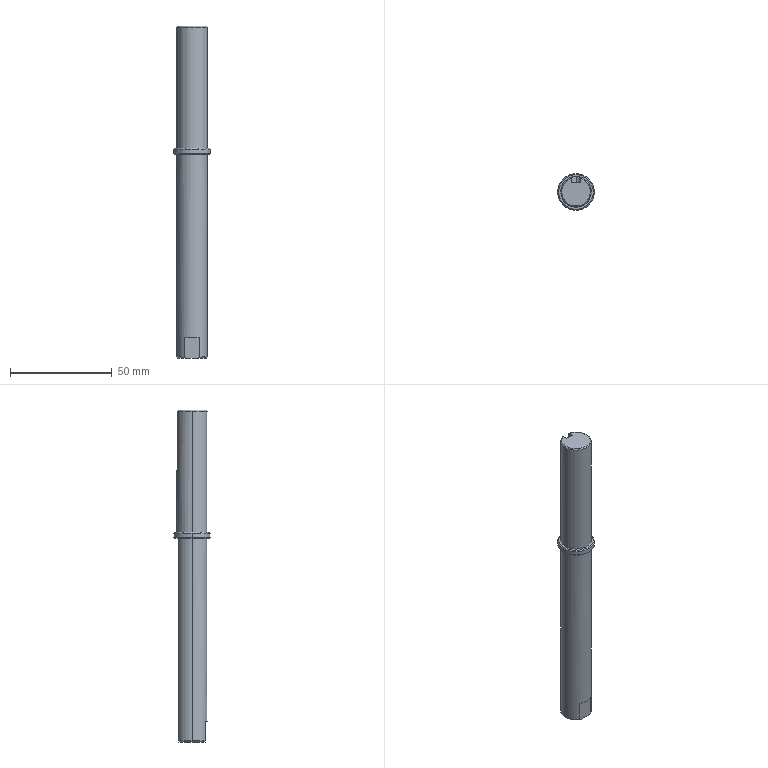Part | STEP file | 10000020500swp000-1 | 1 solid | 29 faces | box 18 x 18 x 163 mm | volume 28114 mm3 | cone 10 | plane 10 | cylinder 9 | commonest cylinder face diameters 15 x5 4 x2 18 x2
STEP:
#1=CARTESIAN_POINT('',(7.,0.,0.));
#2=VERTEX_POINT('',#1);
#3=CARTESIAN_POINT('',(2.,6.708,0.));
#4=VERTEX_POINT('',#3);
#5=CARTESIAN_POINT('',(0.,0.,0.));
#6=DIRECTION('',(0.,0.,1.));
#7=DIRECTION('',(1.,0.,0.));
#8=AXIS2_PLACEMENT_3D('',#5,#6,#7);
#9=CIRCLE('',#8,7.);
#10=EDGE_CURVE('',#2,#4,#9,.T.);
#11=ORIENTED_EDGE('',*,*,#10,.F.);
#12=CARTESIAN_POINT('',(7.5,0.,-0.5));
#13=VERTEX_POINT('',#12);
#14=CARTESIAN_POINT('',(7.,0.,0.));
#15=DIRECTION('',(0.7071,0.,-0.7071));
#16=VECTOR('',#15,1000.);
#17=LINE('',#14,#16);
#18=EDGE_CURVE('',#2,#13,#17,.T.);
#19=ORIENTED_EDGE('',*,*,#18,.T.);
#20=CARTESIAN_POINT('',(2.,7.228,-0.5));
#21=VERTEX_POINT('',#20);
#22=CARTESIAN_POINT('',(0.,0.,-0.5));
#23=DIRECTION('',(0.,0.,-1.));
#24=DIRECTION('',(1.,0.,0.));
#25=AXIS2_PLACEMENT_3D('',#22,#23,#24);
#26=CIRCLE('',#25,7.5);
#27=EDGE_CURVE('',#21,#13,#26,.T.);
#28=ORIENTED_EDGE('',*,*,#27,.F.);
#29=CARTESIAN_POINT('',(2.,6.708,0.));
#30=CARTESIAN_POINT('',(2.,6.882,-0.1664));
#31=CARTESIAN_POINT('',(2.,7.055,-0.3331));
#32=CARTESIAN_POINT('',(2.,7.228,-0.5));
#33=B_SPLINE_CURVE_WITH_KNOTS('',3,(#29,#30,#31,#32),.UNSPECIFIED.,.F.,.F.,(4,4),(0.,0.0007215),.UNSPECIFIED.);
#34=EDGE_CURVE('',#4,#21,#33,.T.);
#35=ORIENTED_EDGE('',*,*,#34,.F.);
#36=EDGE_LOOP('',(#11,#19,#28,#35));
#37=FACE_OUTER_BOUND('',#36,.T.);
#38=CARTESIAN_POINT('',(0.,0.,0.));
#39=DIRECTION('',(0.,0.,-1.));
#40=DIRECTION('',(-1.,0.,0.));
#41=AXIS2_PLACEMENT_3D('',#38,#39,#40);
#42=CONICAL_SURFACE('',#41,7.,0.7854);
#43=ADVANCED_FACE('',(#37),#42,.T.);
#44=ORIENTED_EDGE('',*,*,#18,.F.);
#45=CARTESIAN_POINT('',(-7.,0.,0.));
#46=VERTEX_POINT('',#45);
#47=CARTESIAN_POINT('',(0.,0.,0.));
#48=DIRECTION('',(0.,0.,1.));
#49=DIRECTION('',(1.,0.,0.));
#50=AXIS2_PLACEMENT_3D('',#47,#48,#49);
#51=CIRCLE('',#50,7.);
#52=EDGE_CURVE('',#46,#2,#51,.T.);
#53=ORIENTED_EDGE('',*,*,#52,.F.);
#54=CARTESIAN_POINT('',(-7.5,0.,-0.5));
#55=VERTEX_POINT('',#54);
#56=CARTESIAN_POINT('',(-7.,0.,0.));
#57=DIRECTION('',(-0.7071,0.,-0.7071));
#58=VECTOR('',#57,1000.);
#59=LINE('',#56,#58);
#60=EDGE_CURVE('',#46,#55,#59,.T.);
#61=ORIENTED_EDGE('',*,*,#60,.T.);
#62=CARTESIAN_POINT('',(0.,0.,-0.5));
#63=DIRECTION('',(0.,0.,-1.));
#64=DIRECTION('',(1.,0.,0.));
#65=AXIS2_PLACEMENT_3D('',#62,#63,#64);
#66=CIRCLE('',#65,7.5);
#67=EDGE_CURVE('',#13,#55,#66,.T.);
#68=ORIENTED_EDGE('',*,*,#67,.F.);
#69=EDGE_LOOP('',(#44,#53,#61,#68));
#70=FACE_OUTER_BOUND('',#69,.T.);
#71=CARTESIAN_POINT('',(0.,0.,0.));
#72=DIRECTION('',(0.,0.,-1.));
#73=DIRECTION('',(-1.,0.,0.));
#74=AXIS2_PLACEMENT_3D('',#71,#72,#73);
#75=CONICAL_SURFACE('',#74,7.,0.7854);
#76=ADVANCED_FACE('',(#70),#75,.T.);
#77=CARTESIAN_POINT('',(8.5,0.,-60.));
#78=VERTEX_POINT('',#77);
#79=CARTESIAN_POINT('',(-8.5,0.,-60.));
#80=VERTEX_POINT('',#79);
#81=CARTESIAN_POINT('',(0.,0.,-60.));
#82=DIRECTION('',(0.,0.,1.));
#83=DIRECTION('',(-1.,0.,0.));
#84=AXIS2_PLACEMENT_3D('',#81,#82,#83);
#85=CIRCLE('',#84,8.5);
#86=EDGE_CURVE('',#78,#80,#85,.T.);
#87=ORIENTED_EDGE('',*,*,#86,.F.);
#88=CARTESIAN_POINT('',(9.,0.,-60.5));
#89=VERTEX_POINT('',#88);
#90=CARTESIAN_POINT('',(9.,0.,-60.5));
#91=DIRECTION('',(0.7071,0.,-0.7071));
#92=VECTOR('',#91,1000.);
#93=LINE('',#90,#92);
#94=EDGE_CURVE('',#78,#89,#93,.T.);
#95=ORIENTED_EDGE('',*,*,#94,.T.);
#96=CARTESIAN_POINT('',(-9.,0.,-60.5));
#97=VERTEX_POINT('',#96);
#98=CARTESIAN_POINT('',(0.,0.,-60.5));
#99=DIRECTION('',(0.,0.,-1.));
#100=DIRECTION('',(-1.,0.,0.));
#101=AXIS2_PLACEMENT_3D('',#98,#99,#100);
#102=CIRCLE('',#101,9.);
#103=EDGE_CURVE('',#97,#89,#102,.T.);
#104=ORIENTED_EDGE('',*,*,#103,.F.);
#105=CARTESIAN_POINT('',(-9.,0.,-60.5));
#106=DIRECTION('',(-0.7071,0.,-0.7071));
#107=VECTOR('',#106,1000.);
#108=LINE('',#105,#107);
#109=EDGE_CURVE('',#80,#97,#108,.T.);
#110=ORIENTED_EDGE('',*,*,#109,.F.);
#111=EDGE_LOOP('',(#87,#95,#104,#110));
#112=FACE_OUTER_BOUND('',#111,.T.);
#113=CARTESIAN_POINT('',(0.,0.,-60.5));
#114=DIRECTION('',(0.,0.,-1.));
#115=DIRECTION('',(-1.,0.,0.));
#116=AXIS2_PLACEMENT_3D('',#113,#114,#115);
#117=CONICAL_SURFACE('',#116,9.,0.7854);
#118=ADVANCED_FACE('',(#112),#117,.T.);
#119=CARTESIAN_POINT('',(-8.5,0.,-63.));
#120=VERTEX_POINT('',#119);
#121=CARTESIAN_POINT('',(8.5,0.,-63.));
#122=VERTEX_POINT('',#121);
#123=CARTESIAN_POINT('',(0.,0.,-63.));
#124=DIRECTION('',(0.,0.,-1.));
#125=DIRECTION('',(-1.,0.,0.));
#126=AXIS2_PLACEMENT_3D('',#123,#124,#125);
#127=CIRCLE('',#126,8.5);
#128=EDGE_CURVE('',#120,#122,#127,.T.);
#129=ORIENTED_EDGE('',*,*,#128,.F.);
#130=CARTESIAN_POINT('',(-9.,0.,-62.5));
#131=VERTEX_POINT('',#130);
#132=CARTESIAN_POINT('',(-8.5,0.,-63.));
#133=DIRECTION('',(-0.7071,0.,0.7071));
#134=VECTOR('',#133,1000.);
#135=LINE('',#132,#134);
#136=EDGE_CURVE('',#120,#131,#135,.T.);
#137=ORIENTED_EDGE('',*,*,#136,.T.);
#138=CARTESIAN_POINT('',(9.,0.,-62.5));
#139=VERTEX_POINT('',#138);
#140=CARTESIAN_POINT('',(0.,0.,-62.5));
#141=DIRECTION('',(0.,0.,1.));
#142=DIRECTION('',(-1.,0.,0.));
#143=AXIS2_PLACEMENT_3D('',#140,#141,#142);
#144=CIRCLE('',#143,9.);
#145=EDGE_CURVE('',#139,#131,#144,.T.);
#146=ORIENTED_EDGE('',*,*,#145,.F.);
#147=CARTESIAN_POINT('',(8.5,0.,-63.));
#148=DIRECTION('',(0.7071,0.,0.7071));
#149=VECTOR('',#148,1000.);
#150=LINE('',#147,#149);
#151=EDGE_CURVE('',#122,#139,#150,.T.);
#152=ORIENTED_EDGE('',*,*,#151,.F.);
#153=EDGE_LOOP('',(#129,#137,#146,#152));
#154=FACE_OUTER_BOUND('',#153,.T.);
#155=CARTESIAN_POINT('',(0.,0.,-63.));
#156=DIRECTION('',(0.,0.,1.));
#157=DIRECTION('',(1.,0.,0.));
#158=AXIS2_PLACEMENT_3D('',#155,#156,#157);
#159=CONICAL_SURFACE('',#158,8.5,0.7854);
#160=ADVANCED_FACE('',(#154),#159,.T.);
#161=CARTESIAN_POINT('',(7.,0.,-163.));
#162=VERTEX_POINT('',#161);
#163=CARTESIAN_POINT('',(2.598,-6.5,-163.));
#164=VERTEX_POINT('',#163);
#165=CARTESIAN_POINT('',(0.,0.,-163.));
#166=DIRECTION('',(0.,0.,-1.));
#167=DIRECTION('',(-1.,0.,0.));
#168=AXIS2_PLACEMENT_3D('',#165,#166,#167);
#169=CIRCLE('',#168,7.);
#170=EDGE_CURVE('',#162,#164,#169,.T.);
#171=ORIENTED_EDGE('',*,*,#170,.F.);
#172=CARTESIAN_POINT('',(7.5,0.,-162.5));
#173=VERTEX_POINT('',#172);
#174=CARTESIAN_POINT('',(7.,0.,-163.));
#175=DIRECTION('',(0.7071,0.,0.7071));
#176=VECTOR('',#175,1000.);
#177=LINE('',#174,#176);
#178=EDGE_CURVE('',#162,#173,#177,.T.);
#179=ORIENTED_EDGE('',*,*,#178,.T.);
#180=CARTESIAN_POINT('',(3.742,-6.5,-162.5));
#181=VERTEX_POINT('',#180);
#182=CARTESIAN_POINT('',(0.,0.,-162.5));
#183=DIRECTION('',(0.,0.,1.));
#184=DIRECTION('',(-1.,0.,0.));
#185=AXIS2_PLACEMENT_3D('',#182,#183,#184);
#186=CIRCLE('',#185,7.5);
#187=EDGE_CURVE('',#181,#173,#186,.T.);
#188=ORIENTED_EDGE('',*,*,#187,.F.);
#189=CARTESIAN_POINT('',(2.598,-6.5,-163.));
#190=CARTESIAN_POINT('',(2.991,-6.5,-162.854));
#191=CARTESIAN_POINT('',(3.371,-6.5,-162.685));
#192=CARTESIAN_POINT('',(3.742,-6.5,-162.5));
#193=B_SPLINE_CURVE_WITH_KNOTS('',3,(#189,#190,#191,#192),.UNSPECIFIED.,.F.,.F.,(4,4),(0.02116,0.02241),.UNSPECIFIED.);
#194=EDGE_CURVE('',#164,#181,#193,.T.);
#195=ORIENTED_EDGE('',*,*,#194,.F.);
#196=EDGE_LOOP('',(#171,#179,#188,#195));
#197=FACE_OUTER_BOUND('',#196,.T.);
#198=CARTESIAN_POINT('',(0.,0.,-163.));
#199=DIRECTION('',(0.,0.,1.));
#200=DIRECTION('',(1.,0.,0.));
#201=AXIS2_PLACEMENT_3D('',#198,#199,#200);
#202=CONICAL_SURFACE('',#201,7.,0.7854);
#203=ADVANCED_FACE('',(#197),#202,.T.);
#204=CARTESIAN_POINT('',(0.,7.5,-30.));
#205=VERTEX_POINT('',#204);
#206=CARTESIAN_POINT('',(2.,7.228,-28.));
#207=VERTEX_POINT('',#206);
#208=CARTESIAN_POINT('',(0.,7.5,-30.));
#209=CARTESIAN_POINT('',(0.131,7.5,-30.));
#210=CARTESIAN_POINT('',(0.2641,7.496,-29.987));
#211=CARTESIAN_POINT('',(0.5209,7.483,-29.935));
#212=CARTESIAN_POINT('',(0.6458,7.473,-29.897));
#213=CARTESIAN_POINT('',(1.01,7.436,-29.746));
#214=CARTESIAN_POINT('',(1.229,7.401,-29.599));
#215=CARTESIAN_POINT('',(1.507,7.348,-29.322));
#216=CARTESIAN_POINT('',(1.589,7.33,-29.221));
#217=CARTESIAN_POINT('',(1.734,7.297,-29.006));
#218=CARTESIAN_POINT('',(1.797,7.282,-28.889));
#219=CARTESIAN_POINT('',(1.897,7.256,-28.648));
#220=CARTESIAN_POINT('',(1.935,7.246,-28.523));
#221=CARTESIAN_POINT('',(1.987,7.232,-28.265));
#222=CARTESIAN_POINT('',(2.,7.228,-28.133));
#223=CARTESIAN_POINT('',(2.,7.228,-28.));
#224=B_SPLINE_CURVE_WITH_KNOTS('',3,(#208,#209,#210,#211,#212,#213,#214,#215,#216,#217,#218,#219,#220,#221,#222,#223),.UNSPECIFIED.,.F.,.F.,(4,2,2,2,2,2,2,4),(0.003142,0.003534,0.003926,0.00471,0.005103,0.005495,0.005887,0.006279),.UNSPECIFIED.);
#225=EDGE_CURVE('',#205,#207,#224,.T.);
#226=ORIENTED_EDGE('',*,*,#225,.F.);
#227=CARTESIAN_POINT('',(0.,4.5,-30.));
#228=VERTEX_POINT('',#227);
#229=CARTESIAN_POINT('',(0.,9.,-30.));
#230=DIRECTION('',(0.,-1.,0.));
#231=VECTOR('',#230,1000.);
#232=LINE('',#229,#231);
#233=EDGE_CURVE('',#205,#228,#232,.T.);
#234=ORIENTED_EDGE('',*,*,#233,.T.);
#235=CARTESIAN_POINT('',(2.,4.5,-28.));
#236=VERTEX_POINT('',#235);
#237=CARTESIAN_POINT('',(0.,4.5,-28.));
#238=DIRECTION('',(0.,1.,0.));
#239=DIRECTION('',(0.,0.,1.));
#240=AXIS2_PLACEMENT_3D('',#237,#238,#239);
#241=CIRCLE('',#240,2.);
#242=EDGE_CURVE('',#236,#228,#241,.T.);
#243=ORIENTED_EDGE('',*,*,#242,.F.);
#244=CARTESIAN_POINT('',(2.,9.,-28.));
#245=DIRECTION('',(0.,-1.,0.));
#246=VECTOR('',#245,1000.);
#247=LINE('',#244,#246);
#248=EDGE_CURVE('',#207,#236,#247,.T.);
#249=ORIENTED_EDGE('',*,*,#248,.F.);
#250=EDGE_LOOP('',(#226,#234,#243,#249));
#251=FACE_OUTER_BOUND('',#250,.T.);
#252=CARTESIAN_POINT('',(0.,9.,-28.));
#253=DIRECTION('',(0.,-1.,0.));
#254=DIRECTION('',(0.,0.,-1.));
#255=AXIS2_PLACEMENT_3D('',#252,#253,#254);
#256=CYLINDRICAL_SURFACE('',#255,2.);
#257=ADVANCED_FACE('',(#251),#256,.F.);
#258=ORIENTED_EDGE('',*,*,#145,.T.);
#259=CARTESIAN_POINT('',(-9.,0.,-63.));
#260=DIRECTION('',(0.,0.,1.));
#261=VECTOR('',#260,1000.);
#262=LINE('',#259,#261);
#263=EDGE_CURVE('',#131,#97,#262,.T.);
#264=ORIENTED_EDGE('',*,*,#263,.T.);
#265=ORIENTED_EDGE('',*,*,#103,.T.);
#266=CARTESIAN_POINT('',(9.,0.,-63.));
#267=DIRECTION('',(0.,0.,1.));
#268=VECTOR('',#267,1000.);
#269=LINE('',#266,#268);
#270=EDGE_CURVE('',#139,#89,#269,.T.);
#271=ORIENTED_EDGE('',*,*,#270,.F.);
#272=EDGE_LOOP('',(#258,#264,#265,#271));
#273=FACE_OUTER_BOUND('',#272,.T.);
#274=CARTESIAN_POINT('',(0.,0.,-63.));
#275=DIRECTION('',(0.,0.,1.));
#276=DIRECTION('',(1.,0.,0.));
#277=AXIS2_PLACEMENT_3D('',#274,#275,#276);
#278=CYLINDRICAL_SURFACE('',#277,9.);
#279=ADVANCED_FACE('',(#273),#278,.T.);
#280=CARTESIAN_POINT('',(-3.742,6.5,-162.5));
#281=VERTEX_POINT('',#280);
#282=CARTESIAN_POINT('',(-7.5,0.,-162.5));
#283=VERTEX_POINT('',#282);
#284=CARTESIAN_POINT('',(0.,0.,-162.5));
#285=DIRECTION('',(0.,0.,1.));
#286=DIRECTION('',(-1.,0.,0.));
#287=AXIS2_PLACEMENT_3D('',#284,#285,#286);
#288=CIRCLE('',#287,7.5);
#289=EDGE_CURVE('',#281,#283,#288,.T.);
#290=ORIENTED_EDGE('',*,*,#289,.T.);
#291=CARTESIAN_POINT('',(-7.5,0.,-63.));
#292=VERTEX_POINT('',#291);
#293=CARTESIAN_POINT('',(-7.5,0.,-163.));
#294=DIRECTION('',(0.,0.,1.));
#295=VECTOR('',#294,1000.);
#296=LINE('',#293,#295);
#297=EDGE_CURVE('',#283,#292,#296,.T.);
#298=ORIENTED_EDGE('',*,*,#297,.T.);
#299=CARTESIAN_POINT('',(-3.742,6.5,-63.));
#300=VERTEX_POINT('',#299);
#301=CARTESIAN_POINT('',(0.,0.,-63.));
#302=DIRECTION('',(0.,0.,-1.));
#303=DIRECTION('',(-1.,0.,0.));
#304=AXIS2_PLACEMENT_3D('',#301,#302,#303);
#305=CIRCLE('',#304,7.5);
#306=EDGE_CURVE('',#292,#300,#305,.T.);
#307=ORIENTED_EDGE('',*,*,#306,.T.);
#308=CARTESIAN_POINT('',(-3.742,6.5,-163.));
#309=DIRECTION('',(0.,0.,1.));
#310=VECTOR('',#309,1000.);
#311=LINE('',#308,#310);
#312=EDGE_CURVE('',#281,#300,#311,.T.);
#313=ORIENTED_EDGE('',*,*,#312,.F.);
#314=EDGE_LOOP('',(#290,#298,#307,#313));
#315=FACE_OUTER_BOUND('',#314,.T.);
#316=CARTESIAN_POINT('',(0.,0.,-163.));
#317=DIRECTION('',(0.,0.,1.));
#318=DIRECTION('',(1.,0.,0.));
#319=AXIS2_PLACEMENT_3D('',#316,#317,#318);
#320=CYLINDRICAL_SURFACE('',#319,7.5);
#321=ADVANCED_FACE('',(#315),#320,.T.);
#322=ORIENTED_EDGE('',*,*,#297,.F.);
#323=CARTESIAN_POINT('',(-3.742,-6.5,-162.5));
#324=VERTEX_POINT('',#323);
#325=CARTESIAN_POINT('',(0.,0.,-162.5));
#326=DIRECTION('',(0.,0.,1.));
#327=DIRECTION('',(-1.,0.,0.));
#328=AXIS2_PLACEMENT_3D('',#325,#326,#327);
#329=CIRCLE('',#328,7.5);
#330=EDGE_CURVE('',#283,#324,#329,.T.);
#331=ORIENTED_EDGE('',*,*,#330,.T.);
#332=CARTESIAN_POINT('',(-3.742,-6.5,-153.));
#333=VERTEX_POINT('',#332);
#334=CARTESIAN_POINT('',(-3.742,-6.5,-163.));
#335=DIRECTION('',(0.,0.,1.));
#336=VECTOR('',#335,1000.);
#337=LINE('',#334,#336);
#338=EDGE_CURVE('',#324,#333,#337,.T.);
#339=ORIENTED_EDGE('',*,*,#338,.T.);
#340=CARTESIAN_POINT('',(3.742,-6.5,-153.));
#341=VERTEX_POINT('',#340);
#342=CARTESIAN_POINT('',(0.,0.,-153.));
#343=DIRECTION('',(0.,0.,1.));
#344=DIRECTION('',(1.,0.,0.));
#345=AXIS2_PLACEMENT_3D('',#342,#343,#344);
#346=CIRCLE('',#345,7.5);
#347=EDGE_CURVE('',#333,#341,#346,.T.);
#348=ORIENTED_EDGE('',*,*,#347,.T.);
#349=CARTESIAN_POINT('',(3.742,-6.5,-163.));
#350=DIRECTION('',(0.,0.,-1.));
#351=VECTOR('',#350,1000.);
#352=LINE('',#349,#351);
#353=EDGE_CURVE('',#341,#181,#352,.T.);
#354=ORIENTED_EDGE('',*,*,#353,.T.);
#355=ORIENTED_EDGE('',*,*,#187,.T.);
#356=CARTESIAN_POINT('',(7.5,0.,-63.));
#357=VERTEX_POINT('',#356);
#358=CARTESIAN_POINT('',(7.5,0.,-163.));
#359=DIRECTION('',(0.,0.,1.));
#360=VECTOR('',#359,1000.);
#361=LINE('',#358,#360);
#362=EDGE_CURVE('',#173,#357,#361,.T.);
#363=ORIENTED_EDGE('',*,*,#362,.T.);
#364=CARTESIAN_POINT('',(0.,0.,-63.));
#365=DIRECTION('',(0.,0.,-1.));
#366=DIRECTION('',(-1.,0.,0.));
#367=AXIS2_PLACEMENT_3D('',#364,#365,#366);
#368=CIRCLE('',#367,7.5);
#369=EDGE_CURVE('',#357,#292,#368,.T.);
#370=ORIENTED_EDGE('',*,*,#369,.T.);
#371=EDGE_LOOP('',(#322,#331,#339,#348,#354,#355,#363,#370));
#372=FACE_OUTER_BOUND('',#371,.T.);
#373=CARTESIAN_POINT('',(0.,0.,-163.));
#374=DIRECTION('',(0.,0.,1.));
#375=DIRECTION('',(1.,0.,0.));
#376=AXIS2_PLACEMENT_3D('',#373,#374,#375);
#377=CYLINDRICAL_SURFACE('',#376,7.5);
#378=ADVANCED_FACE('',(#372),#377,.T.);
#379=CARTESIAN_POINT('',(7.5,0.,-60.));
#380=VERTEX_POINT('',#379);
#381=CARTESIAN_POINT('',(-7.5,0.,-60.));
#382=VERTEX_POINT('',#381);
#383=CARTESIAN_POINT('',(0.,0.,-60.));
#384=DIRECTION('',(0.,0.,1.));
#385=DIRECTION('',(-1.,0.,0.));
#386=AXIS2_PLACEMENT_3D('',#383,#384,#385);
#387=CIRCLE('',#386,7.5);
#388=EDGE_CURVE('',#380,#382,#387,.T.);
#389=ORIENTED_EDGE('',*,*,#388,.T.);
#390=CARTESIAN_POINT('',(-7.5,0.,-60.));
#391=DIRECTION('',(0.,0.,1.));
#392=VECTOR('',#391,1000.);
#393=LINE('',#390,#392);
#394=EDGE_CURVE('',#382,#55,#393,.T.);
#395=ORIENTED_EDGE('',*,*,#394,.T.);
#396=CARTESIAN_POINT('',(-2.,7.228,-0.5));
#397=VERTEX_POINT('',#396);
#398=CARTESIAN_POINT('',(0.,0.,-0.5));
#399=DIRECTION('',(0.,0.,-1.));
#400=DIRECTION('',(1.,0.,0.));
#401=AXIS2_PLACEMENT_3D('',#398,#399,#400);
#402=CIRCLE('',#401,7.5);
#403=EDGE_CURVE('',#55,#397,#402,.T.);
#404=ORIENTED_EDGE('',*,*,#403,.T.);
#405=CARTESIAN_POINT('',(-2.,7.228,-28.));
#406=VERTEX_POINT('',#405);
#407=CARTESIAN_POINT('',(-2.,7.228,-60.));
#408=DIRECTION('',(0.,0.,-1.));
#409=VECTOR('',#408,1000.);
#410=LINE('',#407,#409);
#411=EDGE_CURVE('',#397,#406,#410,.T.);
#412=ORIENTED_EDGE('',*,*,#411,.T.);
#413=CARTESIAN_POINT('',(-2.,7.228,-28.));
#414=CARTESIAN_POINT('',(-2.,7.228,-28.133));
#415=CARTESIAN_POINT('',(-1.987,7.232,-28.263));
#416=CARTESIAN_POINT('',(-1.936,7.246,-28.52));
#417=CARTESIAN_POINT('',(-1.897,7.256,-28.647));
#418=CARTESIAN_POINT('',(-1.796,7.282,-28.889));
#419=CARTESIAN_POINT('',(-1.735,7.297,-29.004));
#420=CARTESIAN_POINT('',(-1.59,7.33,-29.221));
#421=CARTESIAN_POINT('',(-1.505,7.348,-29.323));
#422=CARTESIAN_POINT('',(-1.23,7.401,-29.598));
#423=CARTESIAN_POINT('',(-1.008,7.436,-29.747));
#424=CARTESIAN_POINT('',(-0.6467,7.473,-29.897));
#425=CARTESIAN_POINT('',(-0.52,7.483,-29.936));
#426=CARTESIAN_POINT('',(-0.2614,7.497,-29.987));
#427=CARTESIAN_POINT('',(-0.1312,7.5,-30.));
#428=CARTESIAN_POINT('',(0.,7.5,-30.));
#429=B_SPLINE_CURVE_WITH_KNOTS('',3,(#413,#414,#415,#416,#417,#418,#419,#420,#421,#422,#423,#424,#425,#426,#427,#428),.UNSPECIFIED.,.F.,.F.,(4,2,2,2,2,2,2,4),(0.,0.0003927,0.0007854,0.001178,0.001571,0.002356,0.002749,0.003142),.UNSPECIFIED.);
#430=EDGE_CURVE('',#406,#205,#429,.T.);
#431=ORIENTED_EDGE('',*,*,#430,.T.);
#432=ORIENTED_EDGE('',*,*,#225,.T.);
#433=CARTESIAN_POINT('',(2.,7.228,-60.));
#434=DIRECTION('',(0.,0.,1.));
#435=VECTOR('',#434,1000.);
#436=LINE('',#433,#435);
#437=EDGE_CURVE('',#207,#21,#436,.T.);
#438=ORIENTED_EDGE('',*,*,#437,.T.);
#439=ORIENTED_EDGE('',*,*,#27,.T.);
#440=CARTESIAN_POINT('',(7.5,0.,-60.));
#441=DIRECTION('',(0.,0.,1.));
#442=VECTOR('',#441,1000.);
#443=LINE('',#440,#442);
#444=EDGE_CURVE('',#380,#13,#443,.T.);
#445=ORIENTED_EDGE('',*,*,#444,.F.);
#446=EDGE_LOOP('',(#389,#395,#404,#412,#431,#432,#438,#439,#445));
#447=FACE_OUTER_BOUND('',#446,.T.);
#448=CARTESIAN_POINT('',(0.,0.,-60.));
#449=DIRECTION('',(0.,0.,1.));
#450=DIRECTION('',(1.,0.,0.));
#451=AXIS2_PLACEMENT_3D('',#448,#449,#450);
#452=CYLINDRICAL_SURFACE('',#451,7.5);
#453=ADVANCED_FACE('',(#447),#452,.T.);
#454=CARTESIAN_POINT('',(-2.598,-6.5,-163.));
#455=VERTEX_POINT('',#454);
#456=CARTESIAN_POINT('',(-3.742,-6.5,-162.5));
#457=CARTESIAN_POINT('',(-3.369,-6.5,-162.686));
#458=CARTESIAN_POINT('',(-2.989,-6.5,-162.855));
#459=CARTESIAN_POINT('',(-2.598,-6.5,-163.));
#460=B_SPLINE_CURVE_WITH_KNOTS('',3,(#456,#457,#458,#459),.UNSPECIFIED.,.F.,.F.,(4,4),(0.01459,0.01584),.UNSPECIFIED.);
#461=EDGE_CURVE('',#324,#455,#460,.T.);
#462=ORIENTED_EDGE('',*,*,#461,.F.);
#463=ORIENTED_EDGE('',*,*,#330,.F.);
#464=ORIENTED_EDGE('',*,*,#289,.F.);
#465=CARTESIAN_POINT('',(-2.598,6.5,-163.));
#466=VERTEX_POINT('',#465);
#467=CARTESIAN_POINT('',(-2.598,6.5,-163.));
#468=CARTESIAN_POINT('',(-2.989,6.5,-162.855));
#469=CARTESIAN_POINT('',(-3.369,6.5,-162.686));
#470=CARTESIAN_POINT('',(-3.742,6.5,-162.5));
#471=B_SPLINE_CURVE_WITH_KNOTS('',3,(#467,#468,#469,#470),.UNSPECIFIED.,.F.,.F.,(4,4),(0.,0.001248),.UNSPECIFIED.);
#472=EDGE_CURVE('',#466,#281,#471,.T.);
#473=ORIENTED_EDGE('',*,*,#472,.F.);
#474=CARTESIAN_POINT('',(0.,0.,-163.));
#475=DIRECTION('',(0.,0.,-1.));
#476=DIRECTION('',(-1.,0.,0.));
#477=AXIS2_PLACEMENT_3D('',#474,#475,#476);
#478=CIRCLE('',#477,7.);
#479=EDGE_CURVE('',#455,#466,#478,.T.);
#480=ORIENTED_EDGE('',*,*,#479,.F.);
#481=EDGE_LOOP('',(#462,#463,#464,#473,#480));
#482=FACE_OUTER_BOUND('',#481,.T.);
#483=CARTESIAN_POINT('',(0.,0.,-163.));
#484=DIRECTION('',(0.,0.,1.));
#485=DIRECTION('',(1.,0.,0.));
#486=AXIS2_PLACEMENT_3D('',#483,#484,#485);
#487=CONICAL_SURFACE('',#486,7.,0.7854);
#488=ADVANCED_FACE('',(#482),#487,.T.);
#489=ORIENTED_EDGE('',*,*,#394,.F.);
#490=CARTESIAN_POINT('',(0.,0.,-60.));
#491=DIRECTION('',(0.,0.,1.));
#492=DIRECTION('',(-1.,0.,0.));
#493=AXIS2_PLACEMENT_3D('',#490,#491,#492);
#494=CIRCLE('',#493,7.5);
#495=EDGE_CURVE('',#382,#380,#494,.T.);
#496=ORIENTED_EDGE('',*,*,#495,.T.);
#497=ORIENTED_EDGE('',*,*,#444,.T.);
#498=ORIENTED_EDGE('',*,*,#67,.T.);
#499=EDGE_LOOP('',(#489,#496,#497,#498));
#500=FACE_OUTER_BOUND('',#499,.T.);
#501=CARTESIAN_POINT('',(0.,0.,-60.));
#502=DIRECTION('',(0.,0.,1.));
#503=DIRECTION('',(1.,0.,0.));
#504=AXIS2_PLACEMENT_3D('',#501,#502,#503);
#505=CYLINDRICAL_SURFACE('',#504,7.5);
#506=ADVANCED_FACE('',(#500),#505,.T.);
#507=CARTESIAN_POINT('',(-2.,4.5,0.));
#508=VERTEX_POINT('',#507);
#509=CARTESIAN_POINT('',(-2.,6.708,0.));
#510=VERTEX_POINT('',#509);
#511=CARTESIAN_POINT('',(-2.,0.,0.));
#512=DIRECTION('',(0.,1.,0.));
#513=VECTOR('',#512,1000.);
#514=LINE('',#511,#513);
#515=EDGE_CURVE('',#508,#510,#514,.T.);
#516=ORIENTED_EDGE('',*,*,#515,.T.);
#517=CARTESIAN_POINT('',(0.,0.,0.));
#518=DIRECTION('',(0.,0.,1.));
#519=DIRECTION('',(1.,0.,0.));
#520=AXIS2_PLACEMENT_3D('',#517,#518,#519);
#521=CIRCLE('',#520,7.);
#522=EDGE_CURVE('',#510,#46,#521,.T.);
#523=ORIENTED_EDGE('',*,*,#522,.T.);
#524=ORIENTED_EDGE('',*,*,#52,.T.);
#525=ORIENTED_EDGE('',*,*,#10,.T.);
#526=CARTESIAN_POINT('',(2.,4.5,0.));
#527=VERTEX_POINT('',#526);
#528=CARTESIAN_POINT('',(2.,0.,0.));
#529=DIRECTION('',(0.,-1.,0.));
#530=VECTOR('',#529,1000.);
#531=LINE('',#528,#530);
#532=EDGE_CURVE('',#4,#527,#531,.T.);
#533=ORIENTED_EDGE('',*,*,#532,.T.);
#534=CARTESIAN_POINT('',(0.,4.5,0.));
#535=DIRECTION('',(-1.,0.,0.));
#536=VECTOR('',#535,1000.);
#537=LINE('',#534,#536);
#538=EDGE_CURVE('',#527,#508,#537,.T.);
#539=ORIENTED_EDGE('',*,*,#538,.T.);
#540=EDGE_LOOP('',(#516,#523,#524,#525,#533,#539));
#541=FACE_OUTER_BOUND('',#540,.T.);
#542=CARTESIAN_POINT('',(0.,0.,0.));
#543=DIRECTION('',(0.,0.,1.));
#544=DIRECTION('',(1.,0.,0.));
#545=AXIS2_PLACEMENT_3D('',#542,#543,#544);
#546=PLANE('',#545);
#547=ADVANCED_FACE('',(#541),#546,.T.);
#548=ORIENTED_EDGE('',*,*,#362,.F.);
#549=CARTESIAN_POINT('',(3.742,6.5,-162.5));
#550=VERTEX_POINT('',#549);
#551=CARTESIAN_POINT('',(0.,0.,-162.5));
#552=DIRECTION('',(0.,0.,1.));
#553=DIRECTION('',(-1.,0.,0.));
#554=AXIS2_PLACEMENT_3D('',#551,#552,#553);
#555=CIRCLE('',#554,7.5);
#556=EDGE_CURVE('',#173,#550,#555,.T.);
#557=ORIENTED_EDGE('',*,*,#556,.T.);
#558=CARTESIAN_POINT('',(3.742,6.5,-63.));
#559=VERTEX_POINT('',#558);
#560=CARTESIAN_POINT('',(3.742,6.5,-163.));
#561=DIRECTION('',(0.,0.,-1.));
#562=VECTOR('',#561,1000.);
#563=LINE('',#560,#562);
#564=EDGE_CURVE('',#559,#550,#563,.T.);
#565=ORIENTED_EDGE('',*,*,#564,.F.);
#566=CARTESIAN_POINT('',(0.,0.,-63.));
#567=DIRECTION('',(0.,0.,-1.));
#568=DIRECTION('',(-1.,0.,0.));
#569=AXIS2_PLACEMENT_3D('',#566,#567,#568);
#570=CIRCLE('',#569,7.5);
#571=EDGE_CURVE('',#559,#357,#570,.T.);
#572=ORIENTED_EDGE('',*,*,#571,.T.);
#573=EDGE_LOOP('',(#548,#557,#565,#572));
#574=FACE_OUTER_BOUND('',#573,.T.);
#575=CARTESIAN_POINT('',(0.,0.,-163.));
#576=DIRECTION('',(0.,0.,1.));
#577=DIRECTION('',(1.,0.,0.));
#578=AXIS2_PLACEMENT_3D('',#575,#576,#577);
#579=CYLINDRICAL_SURFACE('',#578,7.5);
#580=ADVANCED_FACE('',(#574),#579,.T.);
#581=CARTESIAN_POINT('',(-15.,-6.5,-163.));
#582=DIRECTION('',(1.,0.,0.));
#583=VECTOR('',#582,1000.);
#584=LINE('',#581,#583);
#585=EDGE_CURVE('',#455,#164,#584,.T.);
#586=ORIENTED_EDGE('',*,*,#585,.F.);
#587=ORIENTED_EDGE('',*,*,#479,.T.);
#588=CARTESIAN_POINT('',(2.598,6.5,-163.));
#589=VERTEX_POINT('',#588);
#590=CARTESIAN_POINT('',(0.,6.5,-163.));
#591=DIRECTION('',(1.,0.,0.));
#592=VECTOR('',#591,1000.);
#593=LINE('',#590,#592);
#594=EDGE_CURVE('',#466,#589,#593,.T.);
#595=ORIENTED_EDGE('',*,*,#594,.T.);
#596=CARTESIAN_POINT('',(0.,0.,-163.));
#597=DIRECTION('',(0.,0.,-1.));
#598=DIRECTION('',(-1.,0.,0.));
#599=AXIS2_PLACEMENT_3D('',#596,#597,#598);
#600=CIRCLE('',#599,7.);
#601=EDGE_CURVE('',#589,#162,#600,.T.);
#602=ORIENTED_EDGE('',*,*,#601,.T.);
#603=ORIENTED_EDGE('',*,*,#170,.T.);
#604=EDGE_LOOP('',(#586,#587,#595,#602,#603));
#605=FACE_OUTER_BOUND('',#604,.T.);
#606=CARTESIAN_POINT('',(0.,0.,-163.));
#607=DIRECTION('',(0.,0.,-1.));
#608=DIRECTION('',(-1.,0.,0.));
#609=AXIS2_PLACEMENT_3D('',#606,#607,#608);
#610=PLANE('',#609);
#611=ADVANCED_FACE('',(#605),#610,.T.);
#612=ORIENTED_EDGE('',*,*,#263,.F.);
#613=CARTESIAN_POINT('',(0.,0.,-62.5));
#614=DIRECTION('',(0.,0.,1.));
#615=DIRECTION('',(-1.,0.,0.));
#616=AXIS2_PLACEMENT_3D('',#613,#614,#615);
#617=CIRCLE('',#616,9.);
#618=EDGE_CURVE('',#131,#139,#617,.T.);
#619=ORIENTED_EDGE('',*,*,#618,.T.);
#620=ORIENTED_EDGE('',*,*,#270,.T.);
#621=CARTESIAN_POINT('',(0.,0.,-60.5));
#622=DIRECTION('',(0.,0.,-1.));
#623=DIRECTION('',(-1.,0.,0.));
#624=AXIS2_PLACEMENT_3D('',#621,#622,#623);
#625=CIRCLE('',#624,9.);
#626=EDGE_CURVE('',#89,#97,#625,.T.);
#627=ORIENTED_EDGE('',*,*,#626,.T.);
#628=EDGE_LOOP('',(#612,#619,#620,#627));
#629=FACE_OUTER_BOUND('',#628,.T.);
#630=CARTESIAN_POINT('',(0.,0.,-63.));
#631=DIRECTION('',(0.,0.,1.));
#632=DIRECTION('',(1.,0.,0.));
#633=AXIS2_PLACEMENT_3D('',#630,#631,#632);
#634=CYLINDRICAL_SURFACE('',#633,9.);
#635=ADVANCED_FACE('',(#629),#634,.T.);
#636=CARTESIAN_POINT('',(0.,0.,-63.));
#637=DIRECTION('',(0.,0.,-1.));
#638=DIRECTION('',(-1.,0.,0.));
#639=AXIS2_PLACEMENT_3D('',#636,#637,#638);
#640=CIRCLE('',#639,8.5);
#641=EDGE_CURVE('',#122,#120,#640,.T.);
#642=ORIENTED_EDGE('',*,*,#641,.T.);
#643=ORIENTED_EDGE('',*,*,#128,.T.);
#644=EDGE_LOOP('',(#642,#643));
#645=FACE_OUTER_BOUND('',#644,.T.);
#646=CARTESIAN_POINT('',(-5.,6.5,-63.));
#647=DIRECTION('',(1.,0.,0.));
#648=VECTOR('',#647,1000.);
#649=LINE('',#646,#648);
#650=EDGE_CURVE('',#300,#559,#649,.T.);
#651=ORIENTED_EDGE('',*,*,#650,.F.);
#652=ORIENTED_EDGE('',*,*,#306,.F.);
#653=ORIENTED_EDGE('',*,*,#369,.F.);
#654=ORIENTED_EDGE('',*,*,#571,.F.);
#655=EDGE_LOOP('',(#651,#652,#653,#654));
#656=FACE_BOUND('',#655,.T.);
#657=CARTESIAN_POINT('',(0.,0.,-63.));
#658=DIRECTION('',(0.,0.,-1.));
#659=DIRECTION('',(-1.,0.,0.));
#660=AXIS2_PLACEMENT_3D('',#657,#658,#659);
#661=PLANE('',#660);
#662=ADVANCED_FACE('',(#645,#656),#661,.T.);
#663=CARTESIAN_POINT('',(0.,0.,-60.));
#664=DIRECTION('',(0.,0.,1.));
#665=DIRECTION('',(-1.,0.,0.));
#666=AXIS2_PLACEMENT_3D('',#663,#664,#665);
#667=CIRCLE('',#666,8.5);
#668=EDGE_CURVE('',#80,#78,#667,.T.);
#669=ORIENTED_EDGE('',*,*,#668,.T.);
#670=ORIENTED_EDGE('',*,*,#86,.T.);
#671=EDGE_LOOP('',(#669,#670));
#672=FACE_OUTER_BOUND('',#671,.T.);
#673=ORIENTED_EDGE('',*,*,#388,.F.);
#674=ORIENTED_EDGE('',*,*,#495,.F.);
#675=EDGE_LOOP('',(#673,#674));
#676=FACE_BOUND('',#675,.T.);
#677=CARTESIAN_POINT('',(0.,0.,-60.));
#678=DIRECTION('',(0.,0.,-1.));
#679=DIRECTION('',(-1.,0.,0.));
#680=AXIS2_PLACEMENT_3D('',#677,#678,#679);
#681=PLANE('',#680);
#682=ADVANCED_FACE('',(#672,#676),#681,.F.);
#683=ORIENTED_EDGE('',*,*,#594,.F.);
#684=ORIENTED_EDGE('',*,*,#472,.T.);
#685=ORIENTED_EDGE('',*,*,#312,.T.);
#686=ORIENTED_EDGE('',*,*,#650,.T.);
#687=ORIENTED_EDGE('',*,*,#564,.T.);
#688=CARTESIAN_POINT('',(3.742,6.5,-162.5));
#689=CARTESIAN_POINT('',(3.369,6.5,-162.686));
#690=CARTESIAN_POINT('',(2.989,6.5,-162.855));
#691=CARTESIAN_POINT('',(2.598,6.5,-163.));
#692=B_SPLINE_CURVE_WITH_KNOTS('',3,(#688,#689,#690,#691),.UNSPECIFIED.,.F.,.F.,(4,4),(0.,0.001248),.UNSPECIFIED.);
#693=EDGE_CURVE('',#550,#589,#692,.T.);
#694=ORIENTED_EDGE('',*,*,#693,.T.);
#695=EDGE_LOOP('',(#683,#684,#685,#686,#687,#694));
#696=FACE_OUTER_BOUND('',#695,.T.);
#697=CARTESIAN_POINT('',(0.,6.5,0.));
#698=DIRECTION('',(0.,1.,0.));
#699=DIRECTION('',(0.,0.,1.));
#700=AXIS2_PLACEMENT_3D('',#697,#698,#699);
#701=PLANE('',#700);
#702=ADVANCED_FACE('',(#696),#701,.T.);
#703=ORIENTED_EDGE('',*,*,#532,.F.);
#704=ORIENTED_EDGE('',*,*,#34,.T.);
#705=ORIENTED_EDGE('',*,*,#437,.F.);
#706=ORIENTED_EDGE('',*,*,#248,.T.);
#707=CARTESIAN_POINT('',(2.,4.5,0.));
#708=DIRECTION('',(0.,0.,-1.));
#709=VECTOR('',#708,1000.);
#710=LINE('',#707,#709);
#711=EDGE_CURVE('',#527,#236,#710,.T.);
#712=ORIENTED_EDGE('',*,*,#711,.F.);
#713=EDGE_LOOP('',(#703,#704,#705,#706,#712));
#714=FACE_OUTER_BOUND('',#713,.T.);
#715=CARTESIAN_POINT('',(2.,9.,0.));
#716=DIRECTION('',(-1.,0.,0.));
#717=DIRECTION('',(0.,0.,1.));
#718=AXIS2_PLACEMENT_3D('',#715,#716,#717);
#719=PLANE('',#718);
#720=ADVANCED_FACE('',(#714),#719,.T.);
#721=ORIENTED_EDGE('',*,*,#233,.F.);
#722=ORIENTED_EDGE('',*,*,#430,.F.);
#723=CARTESIAN_POINT('',(-2.,4.5,-28.));
#724=VERTEX_POINT('',#723);
#725=CARTESIAN_POINT('',(-2.,9.,-28.));
#726=DIRECTION('',(0.,-1.,0.));
#727=VECTOR('',#726,1000.);
#728=LINE('',#725,#727);
#729=EDGE_CURVE('',#406,#724,#728,.T.);
#730=ORIENTED_EDGE('',*,*,#729,.T.);
#731=CARTESIAN_POINT('',(0.,4.5,-28.));
#732=DIRECTION('',(0.,1.,0.));
#733=DIRECTION('',(0.,0.,1.));
#734=AXIS2_PLACEMENT_3D('',#731,#732,#733);
#735=CIRCLE('',#734,2.);
#736=EDGE_CURVE('',#228,#724,#735,.T.);
#737=ORIENTED_EDGE('',*,*,#736,.F.);
#738=EDGE_LOOP('',(#721,#722,#730,#737));
#739=FACE_OUTER_BOUND('',#738,.T.);
#740=CARTESIAN_POINT('',(0.,9.,-28.));
#741=DIRECTION('',(0.,-1.,0.));
#742=DIRECTION('',(0.,0.,-1.));
#743=AXIS2_PLACEMENT_3D('',#740,#741,#742);
#744=CYLINDRICAL_SURFACE('',#743,2.);
#745=ADVANCED_FACE('',(#739),#744,.F.);
#746=ORIENTED_EDGE('',*,*,#411,.F.);
#747=CARTESIAN_POINT('',(-2.,7.228,-0.5));
#748=CARTESIAN_POINT('',(-2.,7.055,-0.3331));
#749=CARTESIAN_POINT('',(-2.,6.882,-0.1664));
#750=CARTESIAN_POINT('',(-2.,6.708,0.));
#751=B_SPLINE_CURVE_WITH_KNOTS('',3,(#747,#748,#749,#750),.UNSPECIFIED.,.F.,.F.,(4,4),(0.,0.0007215),.UNSPECIFIED.);
#752=EDGE_CURVE('',#397,#510,#751,.T.);
#753=ORIENTED_EDGE('',*,*,#752,.T.);
#754=ORIENTED_EDGE('',*,*,#515,.F.);
#755=CARTESIAN_POINT('',(-2.,4.5,0.));
#756=DIRECTION('',(0.,0.,1.));
#757=VECTOR('',#756,1000.);
#758=LINE('',#755,#757);
#759=EDGE_CURVE('',#724,#508,#758,.T.);
#760=ORIENTED_EDGE('',*,*,#759,.F.);
#761=ORIENTED_EDGE('',*,*,#729,.F.);
#762=EDGE_LOOP('',(#746,#753,#754,#760,#761));
#763=FACE_OUTER_BOUND('',#762,.T.);
#764=CARTESIAN_POINT('',(-2.,9.,0.));
#765=DIRECTION('',(1.,0.,0.));
#766=DIRECTION('',(0.,0.,-1.));
#767=AXIS2_PLACEMENT_3D('',#764,#765,#766);
#768=PLANE('',#767);
#769=ADVANCED_FACE('',(#763),#768,.T.);
#770=ORIENTED_EDGE('',*,*,#711,.T.);
#771=ORIENTED_EDGE('',*,*,#242,.T.);
#772=ORIENTED_EDGE('',*,*,#736,.T.);
#773=ORIENTED_EDGE('',*,*,#759,.T.);
#774=ORIENTED_EDGE('',*,*,#538,.F.);
#775=EDGE_LOOP('',(#770,#771,#772,#773,#774));
#776=FACE_OUTER_BOUND('',#775,.T.);
#777=CARTESIAN_POINT('',(0.,4.5,0.));
#778=DIRECTION('',(0.,1.,0.));
#779=DIRECTION('',(0.,0.,1.));
#780=AXIS2_PLACEMENT_3D('',#777,#778,#779);
#781=PLANE('',#780);
#782=ADVANCED_FACE('',(#776),#781,.T.);
#783=ORIENTED_EDGE('',*,*,#178,.F.);
#784=ORIENTED_EDGE('',*,*,#601,.F.);
#785=ORIENTED_EDGE('',*,*,#693,.F.);
#786=ORIENTED_EDGE('',*,*,#556,.F.);
#787=EDGE_LOOP('',(#783,#784,#785,#786));
#788=FACE_OUTER_BOUND('',#787,.T.);
#789=CARTESIAN_POINT('',(0.,0.,-163.));
#790=DIRECTION('',(0.,0.,1.));
#791=DIRECTION('',(1.,0.,0.));
#792=AXIS2_PLACEMENT_3D('',#789,#790,#791);
#793=CONICAL_SURFACE('',#792,7.,0.7854);
#794=ADVANCED_FACE('',(#788),#793,.T.);
#795=ORIENTED_EDGE('',*,*,#136,.F.);
#796=ORIENTED_EDGE('',*,*,#641,.F.);
#797=ORIENTED_EDGE('',*,*,#151,.T.);
#798=ORIENTED_EDGE('',*,*,#618,.F.);
#799=EDGE_LOOP('',(#795,#796,#797,#798));
#800=FACE_OUTER_BOUND('',#799,.T.);
#801=CARTESIAN_POINT('',(0.,0.,-63.));
#802=DIRECTION('',(0.,0.,1.));
#803=DIRECTION('',(1.,0.,0.));
#804=AXIS2_PLACEMENT_3D('',#801,#802,#803);
#805=CONICAL_SURFACE('',#804,8.5,0.7854);
#806=ADVANCED_FACE('',(#800),#805,.T.);
#807=ORIENTED_EDGE('',*,*,#94,.F.);
#808=ORIENTED_EDGE('',*,*,#668,.F.);
#809=ORIENTED_EDGE('',*,*,#109,.T.);
#810=ORIENTED_EDGE('',*,*,#626,.F.);
#811=EDGE_LOOP('',(#807,#808,#809,#810));
#812=FACE_OUTER_BOUND('',#811,.T.);
#813=CARTESIAN_POINT('',(0.,0.,-60.5));
#814=DIRECTION('',(0.,0.,-1.));
#815=DIRECTION('',(-1.,0.,0.));
#816=AXIS2_PLACEMENT_3D('',#813,#814,#815);
#817=CONICAL_SURFACE('',#816,9.,0.7854);
#818=ADVANCED_FACE('',(#812),#817,.T.);
#819=ORIENTED_EDGE('',*,*,#60,.F.);
#820=ORIENTED_EDGE('',*,*,#522,.F.);
#821=ORIENTED_EDGE('',*,*,#752,.F.);
#822=ORIENTED_EDGE('',*,*,#403,.F.);
#823=EDGE_LOOP('',(#819,#820,#821,#822));
#824=FACE_OUTER_BOUND('',#823,.T.);
#825=CARTESIAN_POINT('',(0.,0.,0.));
#826=DIRECTION('',(0.,0.,-1.));
#827=DIRECTION('',(-1.,0.,0.));
#828=AXIS2_PLACEMENT_3D('',#825,#826,#827);
#829=CONICAL_SURFACE('',#828,7.,0.7854);
#830=ADVANCED_FACE('',(#824),#829,.T.);
#831=CARTESIAN_POINT('',(-15.,-6.5,-153.));
#832=DIRECTION('',(1.,0.,0.));
#833=VECTOR('',#832,1000.);
#834=LINE('',#831,#833);
#835=EDGE_CURVE('',#333,#341,#834,.T.);
#836=ORIENTED_EDGE('',*,*,#835,.T.);
#837=ORIENTED_EDGE('',*,*,#347,.F.);
#838=EDGE_LOOP('',(#836,#837));
#839=FACE_OUTER_BOUND('',#838,.T.);
#840=CARTESIAN_POINT('',(-15.,-7.5,-153.));
#841=DIRECTION('',(0.,0.,1.));
#842=DIRECTION('',(1.,0.,0.));
#843=AXIS2_PLACEMENT_3D('',#840,#841,#842);
#844=PLANE('',#843);
#845=ADVANCED_FACE('',(#839),#844,.F.);
#846=ORIENTED_EDGE('',*,*,#461,.T.);
#847=ORIENTED_EDGE('',*,*,#585,.T.);
#848=ORIENTED_EDGE('',*,*,#194,.T.);
#849=ORIENTED_EDGE('',*,*,#353,.F.);
#850=ORIENTED_EDGE('',*,*,#835,.F.);
#851=ORIENTED_EDGE('',*,*,#338,.F.);
#852=EDGE_LOOP('',(#846,#847,#848,#849,#850,#851));
#853=FACE_OUTER_BOUND('',#852,.T.);
#854=CARTESIAN_POINT('',(-15.,-6.5,-153.));
#855=DIRECTION('',(0.,1.,0.));
#856=DIRECTION('',(0.,0.,1.));
#857=AXIS2_PLACEMENT_3D('',#854,#855,#856);
#858=PLANE('',#857);
#859=ADVANCED_FACE('',(#853),#858,.F.);
#860=CLOSED_SHELL('',(#43,#76,#118,#160,#203,#257,#279,#321,#378,#453,#488,#506,#547,#580,#611,#635,#662,#682,#702,#720,#745,#769,#782,#794,#806,#818,#830,#845,#859));
#861=MANIFOLD_SOLID_BREP('',#860);
#862=CARTESIAN_POINT('',(0.,0.,0.));
#863=DIRECTION('',(0.,0.,1.));
#864=DIRECTION('',(1.,0.,0.));
#865=AXIS2_PLACEMENT_3D('',#862,#863,#864);
#866=(LENGTH_UNIT()NAMED_UNIT(*)SI_UNIT(.MILLI.,.METRE.));
#867=UNCERTAINTY_MEASURE_WITH_UNIT(LENGTH_MEASURE(0.00001),#866,'','');
#868=(NAMED_UNIT(*)PLANE_ANGLE_UNIT()SI_UNIT($,.RADIAN.));
#869=(NAMED_UNIT(*)SI_UNIT($,.STERADIAN.)SOLID_ANGLE_UNIT());
#870=(GEOMETRIC_REPRESENTATION_CONTEXT(3)GLOBAL_UNCERTAINTY_ASSIGNED_CONTEXT((#867))GLOBAL_UNIT_ASSIGNED_CONTEXT((#866,#868,#869))REPRESENTATION_CONTEXT('',''));
#871=ADVANCED_BREP_SHAPE_REPRESENTATION('',(#861,#865),#870);